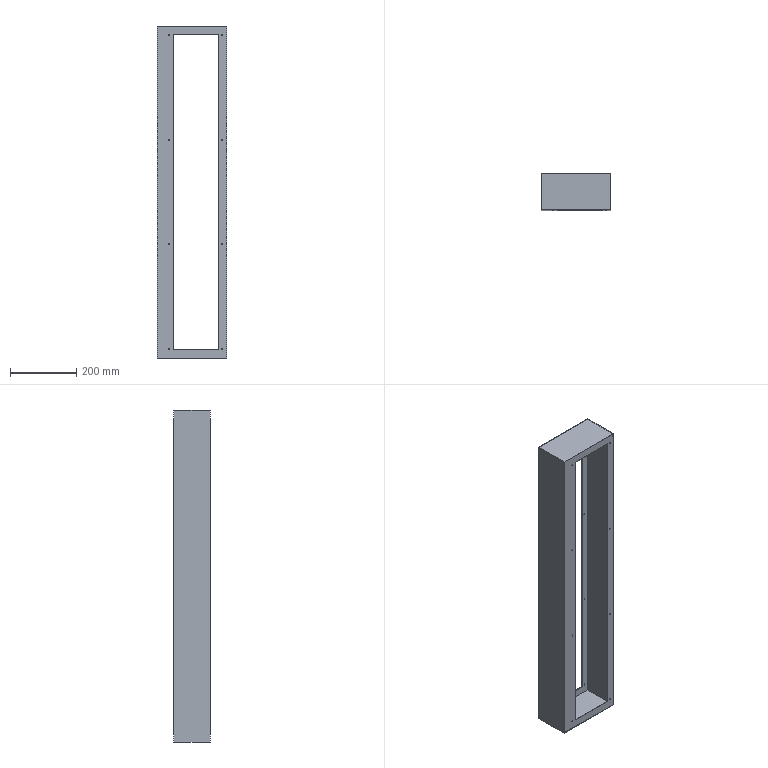Part | STEP file | 1 solid | 52 faces | box 210 x 110 x 1000 mm | volume 594029 mm3 | cylinder 32 | plane 20 | commonest cylinder face diameters 3.2 x32